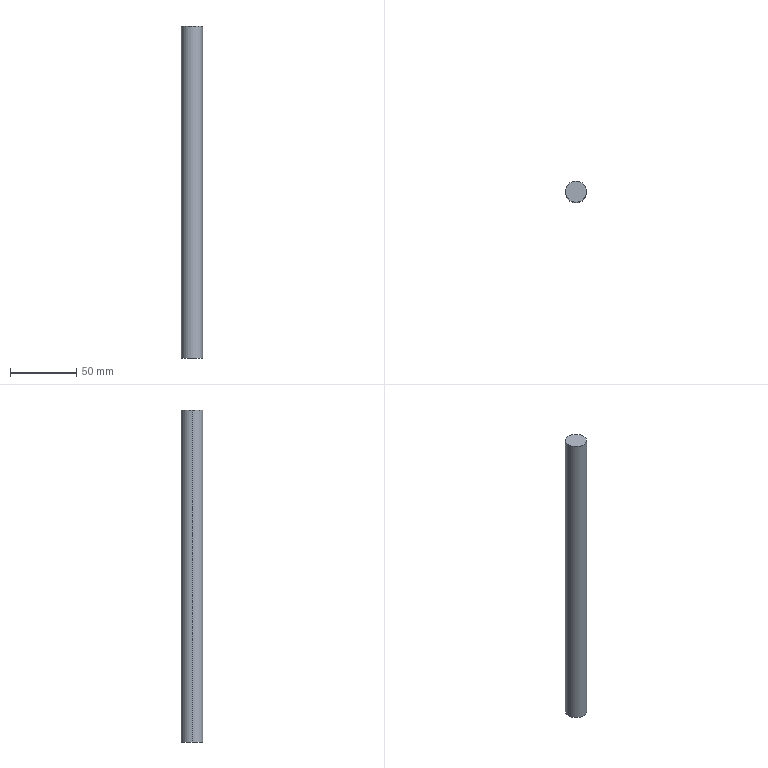Part | SolidWorks | features Extrusion 1 | 1 solid | 4 faces | box 16 x 16 x 250 mm | volume 50265 mm3 | cylinder 2 | plane 2 | commonest cylinder face diameters 16 x2
STEP:
#1=CARTESIAN_POINT('',(8.,0.,250.));
#2=VERTEX_POINT('',#1);
#3=CARTESIAN_POINT('',(-8.,0.,250.));
#4=VERTEX_POINT('',#3);
#5=CARTESIAN_POINT('',(0.,0.,250.));
#6=DIRECTION('',(0.,0.,1.));
#7=DIRECTION('',(1.,0.,0.));
#8=AXIS2_PLACEMENT_3D('',#5,#6,#7);
#9=CIRCLE('',#8,8.);
#10=EDGE_CURVE('',#2,#4,#9,.T.);
#11=ORIENTED_EDGE('',*,*,#10,.F.);
#12=CARTESIAN_POINT('',(8.,0.,0.));
#13=VERTEX_POINT('',#12);
#14=CARTESIAN_POINT('',(8.,0.,250.));
#15=DIRECTION('',(0.,0.,-1.));
#16=VECTOR('',#15,1000.);
#17=LINE('',#14,#16);
#18=EDGE_CURVE('',#2,#13,#17,.T.);
#19=ORIENTED_EDGE('',*,*,#18,.T.);
#20=CARTESIAN_POINT('',(-8.,0.,0.));
#21=VERTEX_POINT('',#20);
#22=CARTESIAN_POINT('',(0.,0.,0.));
#23=DIRECTION('',(0.,0.,1.));
#24=DIRECTION('',(1.,0.,0.));
#25=AXIS2_PLACEMENT_3D('',#22,#23,#24);
#26=CIRCLE('',#25,8.);
#27=EDGE_CURVE('',#13,#21,#26,.T.);
#28=ORIENTED_EDGE('',*,*,#27,.T.);
#29=CARTESIAN_POINT('',(-8.,0.,250.));
#30=DIRECTION('',(0.,0.,-1.));
#31=VECTOR('',#30,1000.);
#32=LINE('',#29,#31);
#33=EDGE_CURVE('',#4,#21,#32,.T.);
#34=ORIENTED_EDGE('',*,*,#33,.F.);
#35=EDGE_LOOP('',(#11,#19,#28,#34));
#36=FACE_OUTER_BOUND('',#35,.T.);
#37=CARTESIAN_POINT('',(0.,0.,250.));
#38=DIRECTION('',(0.,0.,-1.));
#39=DIRECTION('',(-1.,0.,0.));
#40=AXIS2_PLACEMENT_3D('',#37,#38,#39);
#41=CYLINDRICAL_SURFACE('',#40,8.);
#42=ADVANCED_FACE('',(#36),#41,.T.);
#43=ORIENTED_EDGE('',*,*,#18,.F.);
#44=CARTESIAN_POINT('',(0.,0.,250.));
#45=DIRECTION('',(0.,0.,1.));
#46=DIRECTION('',(1.,0.,0.));
#47=AXIS2_PLACEMENT_3D('',#44,#45,#46);
#48=CIRCLE('',#47,8.);
#49=EDGE_CURVE('',#4,#2,#48,.T.);
#50=ORIENTED_EDGE('',*,*,#49,.F.);
#51=ORIENTED_EDGE('',*,*,#33,.T.);
#52=CARTESIAN_POINT('',(0.,0.,0.));
#53=DIRECTION('',(0.,0.,1.));
#54=DIRECTION('',(1.,0.,0.));
#55=AXIS2_PLACEMENT_3D('',#52,#53,#54);
#56=CIRCLE('',#55,8.);
#57=EDGE_CURVE('',#21,#13,#56,.T.);
#58=ORIENTED_EDGE('',*,*,#57,.T.);
#59=EDGE_LOOP('',(#43,#50,#51,#58));
#60=FACE_OUTER_BOUND('',#59,.T.);
#61=CARTESIAN_POINT('',(0.,0.,250.));
#62=DIRECTION('',(0.,0.,-1.));
#63=DIRECTION('',(-1.,0.,0.));
#64=AXIS2_PLACEMENT_3D('',#61,#62,#63);
#65=CYLINDRICAL_SURFACE('',#64,8.);
#66=ADVANCED_FACE('',(#60),#65,.T.);
#67=ORIENTED_EDGE('',*,*,#49,.T.);
#68=ORIENTED_EDGE('',*,*,#10,.T.);
#69=EDGE_LOOP('',(#67,#68));
#70=FACE_OUTER_BOUND('',#69,.T.);
#71=CARTESIAN_POINT('',(0.,0.,250.));
#72=DIRECTION('',(0.,0.,1.));
#73=DIRECTION('',(1.,0.,0.));
#74=AXIS2_PLACEMENT_3D('',#71,#72,#73);
#75=PLANE('',#74);
#76=ADVANCED_FACE('',(#70),#75,.T.);
#77=ORIENTED_EDGE('',*,*,#57,.F.);
#78=ORIENTED_EDGE('',*,*,#27,.F.);
#79=EDGE_LOOP('',(#77,#78));
#80=FACE_OUTER_BOUND('',#79,.T.);
#81=CARTESIAN_POINT('',(0.,0.,0.));
#82=DIRECTION('',(0.,0.,1.));
#83=DIRECTION('',(1.,0.,0.));
#84=AXIS2_PLACEMENT_3D('',#81,#82,#83);
#85=PLANE('',#84);
#86=ADVANCED_FACE('',(#80),#85,.F.);
#87=CLOSED_SHELL('',(#42,#66,#76,#86));
#88=MANIFOLD_SOLID_BREP('',#87);
#89=CARTESIAN_POINT('',(0.,0.,0.));
#90=DIRECTION('',(0.,0.,1.));
#91=DIRECTION('',(1.,0.,0.));
#92=AXIS2_PLACEMENT_3D('',#89,#90,#91);
#93=(LENGTH_UNIT()NAMED_UNIT(*)SI_UNIT(.MILLI.,.METRE.));
#94=UNCERTAINTY_MEASURE_WITH_UNIT(LENGTH_MEASURE(0.00001),#93,'','');
#95=(NAMED_UNIT(*)PLANE_ANGLE_UNIT()SI_UNIT($,.RADIAN.));
#96=(NAMED_UNIT(*)SI_UNIT($,.STERADIAN.)SOLID_ANGLE_UNIT());
#97=(GEOMETRIC_REPRESENTATION_CONTEXT(3)GLOBAL_UNCERTAINTY_ASSIGNED_CONTEXT((#94))GLOBAL_UNIT_ASSIGNED_CONTEXT((#93,#95,#96))REPRESENTATION_CONTEXT('',''));
#98=ADVANCED_BREP_SHAPE_REPRESENTATION('',(#88,#92),#97);